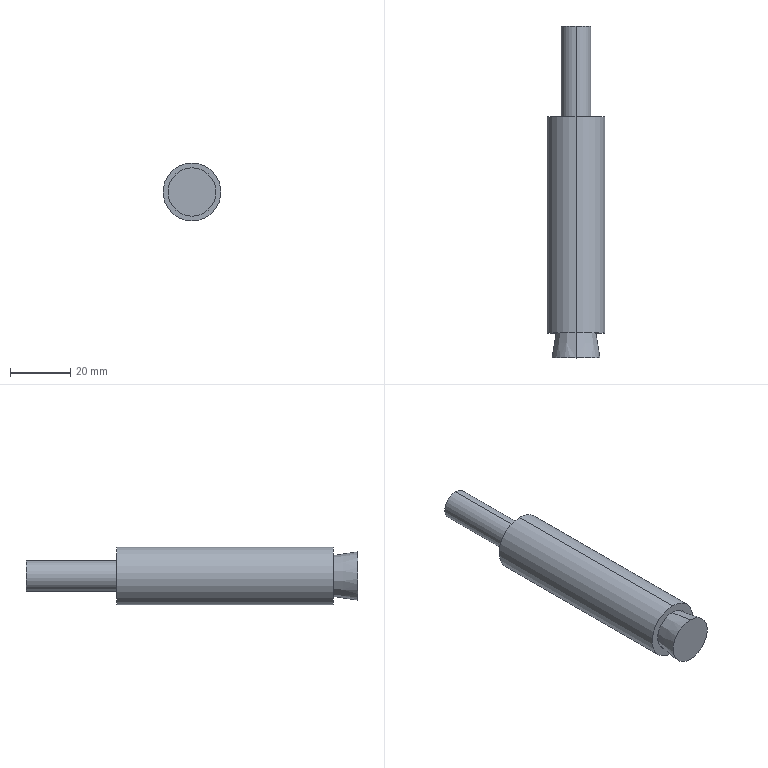Part | STEP file | Expansion Bolt M10X110 | 2 solids | 12 faces | box 19.178 x 110 x 19.178 mm | volume 19450 mm3 | cylinder 6 | plane 4 | cone 2 | commonest cylinder face diameters 10 x2 14 x2 19.178 x2
STEP:
#1=CARTESIAN_POINT('',(0.,0.,0.));
#2=DIRECTION('',(0.,0.,1.));
#3=DIRECTION('',(1.,0.,0.));
#4=AXIS2_PLACEMENT_3D('',#1,#2,#3);
#5=CARTESIAN_POINT('',(0.,110.,-5.));
#6=VERTEX_POINT('',#5);
#7=CARTESIAN_POINT('',(0.,110.,5.));
#8=VERTEX_POINT('',#7);
#9=CARTESIAN_POINT('',(0.,110.,0.));
#10=DIRECTION('',(0.,-1.,0.));
#11=DIRECTION('',(0.,0.,-1.));
#12=AXIS2_PLACEMENT_3D('',#9,#10,#11);
#13=CIRCLE('',#12,5.);
#14=CARTESIAN_POINT('',(0.,0.,0.));
#15=DIRECTION('',(0.,-1.,0.));
#16=DIRECTION('',(0.,0.,-1.));
#17=AXIS2_PLACEMENT_3D('',#14,#15,#16);
#18=CYLINDRICAL_SURFACE('',#17,5.);
#19=CARTESIAN_POINT('',(0.,-110.));
#20=DIRECTION('',(1.,0.));
#21=VECTOR('',#20,1.);
#22=LINE('',#19,#21);
#23=(GEOMETRIC_REPRESENTATION_CONTEXT(2)PARAMETRIC_REPRESENTATION_CONTEXT()REPRESENTATION_CONTEXT('',''));
#24=DEFINITIONAL_REPRESENTATION('',(#22),#23);
#25=PCURVE('',#18,#24);
#26=CARTESIAN_POINT('',(0.,110.,0.));
#27=DIRECTION('',(0.,1.,0.));
#28=DIRECTION('',(0.,0.,1.));
#29=AXIS2_PLACEMENT_3D('',#26,#27,#28);
#30=PLANE('',#29);
#31=CARTESIAN_POINT('',(-5.,0.));
#32=CARTESIAN_POINT('',(-5.,8.66));
#33=CARTESIAN_POINT('',(2.5,4.33));
#34=CARTESIAN_POINT('',(10.,0.));
#35=CARTESIAN_POINT('',(2.5,-4.33));
#36=CARTESIAN_POINT('',(-5.,-8.66));
#37=CARTESIAN_POINT('',(-5.,0.));
#38=(BOUNDED_CURVE()B_SPLINE_CURVE(2,(#31,#32,#33,#34,#35,#36,#37),.UNSPECIFIED.,.T.,.F.)B_SPLINE_CURVE_WITH_KNOTS((1,2,2,2,2,1),(-2.094,0.,2.094,4.189,6.283,8.378),.UNSPECIFIED.)CURVE()GEOMETRIC_REPRESENTATION_ITEM()RATIONAL_B_SPLINE_CURVE((1.,0.5,1.,0.5,1.,0.5,1.))REPRESENTATION_ITEM(''));
#39=(GEOMETRIC_REPRESENTATION_CONTEXT(2)PARAMETRIC_REPRESENTATION_CONTEXT()REPRESENTATION_CONTEXT('',''));
#40=DEFINITIONAL_REPRESENTATION('',(#38),#39);
#41=PCURVE('',#30,#40);
#42=SURFACE_CURVE('',#13,(#25,#41),.PCURVE_S1.);
#43=EDGE_CURVE('',#6,#8,#42,.T.);
#44=ORIENTED_EDGE('',*,*,#43,.T.);
#45=CARTESIAN_POINT('',(0.,20.,5.));
#46=VERTEX_POINT('',#45);
#47=CARTESIAN_POINT('',(0.,0.,5.));
#48=DIRECTION('',(0.,-1.,0.));
#49=VECTOR('',#48,1.);
#50=LINE('',#47,#49);
#51=CARTESIAN_POINT('',(3.142,0.));
#52=DIRECTION('',(0.,1.));
#53=VECTOR('',#52,1.);
#54=LINE('',#51,#53);
#55=(GEOMETRIC_REPRESENTATION_CONTEXT(2)PARAMETRIC_REPRESENTATION_CONTEXT()REPRESENTATION_CONTEXT('',''));
#56=DEFINITIONAL_REPRESENTATION('',(#54),#55);
#57=PCURVE('',#18,#56);
#58=CARTESIAN_POINT('',(0.,0.,0.));
#59=DIRECTION('',(0.,-1.,0.));
#60=DIRECTION('',(0.,0.,-1.));
#61=AXIS2_PLACEMENT_3D('',#58,#59,#60);
#62=CYLINDRICAL_SURFACE('',#61,5.);
#63=CARTESIAN_POINT('',(3.142,0.));
#64=DIRECTION('',(0.,1.));
#65=VECTOR('',#64,1.);
#66=LINE('',#63,#65);
#67=(GEOMETRIC_REPRESENTATION_CONTEXT(2)PARAMETRIC_REPRESENTATION_CONTEXT()REPRESENTATION_CONTEXT('',''));
#68=DEFINITIONAL_REPRESENTATION('',(#66),#67);
#69=PCURVE('',#62,#68);
#70=SURFACE_CURVE('',#50,(#57,#69),.PCURVE_S1.);
#71=EDGE_CURVE('',#8,#46,#70,.T.);
#72=ORIENTED_EDGE('',*,*,#71,.T.);
#73=CARTESIAN_POINT('',(0.,20.,-5.));
#74=VERTEX_POINT('',#73);
#75=CARTESIAN_POINT('',(0.,20.,0.));
#76=DIRECTION('',(0.,-1.,0.));
#77=DIRECTION('',(0.,0.,-1.));
#78=AXIS2_PLACEMENT_3D('',#75,#76,#77);
#79=CIRCLE('',#78,5.);
#80=CARTESIAN_POINT('',(0.,-20.));
#81=DIRECTION('',(1.,0.));
#82=VECTOR('',#81,1.);
#83=LINE('',#80,#82);
#84=(GEOMETRIC_REPRESENTATION_CONTEXT(2)PARAMETRIC_REPRESENTATION_CONTEXT()REPRESENTATION_CONTEXT('',''));
#85=DEFINITIONAL_REPRESENTATION('',(#83),#84);
#86=PCURVE('',#18,#85);
#87=CARTESIAN_POINT('',(0.,0.,0.));
#88=DIRECTION('',(0.,-1.,0.));
#89=DIRECTION('',(0.,0.,-1.));
#90=AXIS2_PLACEMENT_3D('',#87,#88,#89);
#91=CONICAL_SURFACE('',#90,8.,0.1489);
#92=CARTESIAN_POINT('',(0.,-20.));
#93=DIRECTION('',(1.,0.));
#94=VECTOR('',#93,1.);
#95=LINE('',#92,#94);
#96=(GEOMETRIC_REPRESENTATION_CONTEXT(2)PARAMETRIC_REPRESENTATION_CONTEXT()REPRESENTATION_CONTEXT('',''));
#97=DEFINITIONAL_REPRESENTATION('',(#95),#96);
#98=PCURVE('',#91,#97);
#99=SURFACE_CURVE('',#79,(#86,#98),.PCURVE_S1.);
#100=EDGE_CURVE('',#74,#46,#99,.T.);
#101=ORIENTED_EDGE('',*,*,#100,.F.);
#102=CARTESIAN_POINT('',(0.,0.,-5.));
#103=DIRECTION('',(0.,-1.,0.));
#104=VECTOR('',#103,1.);
#105=LINE('',#102,#104);
#106=CARTESIAN_POINT('',(0.,0.));
#107=DIRECTION('',(0.,1.));
#108=VECTOR('',#107,1.);
#109=LINE('',#106,#108);
#110=(GEOMETRIC_REPRESENTATION_CONTEXT(2)PARAMETRIC_REPRESENTATION_CONTEXT()REPRESENTATION_CONTEXT('',''));
#111=DEFINITIONAL_REPRESENTATION('',(#109),#110);
#112=PCURVE('',#18,#111);
#113=CARTESIAN_POINT('',(6.283,0.));
#114=DIRECTION('',(0.,1.));
#115=VECTOR('',#114,1.);
#116=LINE('',#113,#115);
#117=(GEOMETRIC_REPRESENTATION_CONTEXT(2)PARAMETRIC_REPRESENTATION_CONTEXT()REPRESENTATION_CONTEXT('',''));
#118=DEFINITIONAL_REPRESENTATION('',(#116),#117);
#119=PCURVE('',#62,#118);
#120=SURFACE_CURVE('',#105,(#112,#119),.PCURVE_S1.);
#121=EDGE_CURVE('',#6,#74,#120,.T.);
#122=ORIENTED_EDGE('',*,*,#121,.F.);
#123=EDGE_LOOP('',(#44,#72,#101,#122));
#124=FACE_BOUND('',#123,.T.);
#125=ADVANCED_FACE('',(#124),#18,.T.);
#126=ORIENTED_EDGE('',*,*,#100,.T.);
#127=CARTESIAN_POINT('',(0.,0.,8.));
#128=VERTEX_POINT('',#127);
#129=CARTESIAN_POINT('',(0.,0.,8.));
#130=DIRECTION('',(0.,-0.9889,0.1483));
#131=VECTOR('',#130,1.);
#132=LINE('',#129,#131);
#133=CARTESIAN_POINT('',(3.142,0.));
#134=DIRECTION('',(0.,1.));
#135=VECTOR('',#134,1.);
#136=LINE('',#133,#135);
#137=(GEOMETRIC_REPRESENTATION_CONTEXT(2)PARAMETRIC_REPRESENTATION_CONTEXT()REPRESENTATION_CONTEXT('',''));
#138=DEFINITIONAL_REPRESENTATION('',(#136),#137);
#139=PCURVE('',#91,#138);
#140=CARTESIAN_POINT('',(0.,0.,0.));
#141=DIRECTION('',(0.,-1.,0.));
#142=DIRECTION('',(0.,0.,-1.));
#143=AXIS2_PLACEMENT_3D('',#140,#141,#142);
#144=CONICAL_SURFACE('',#143,8.,0.1489);
#145=CARTESIAN_POINT('',(3.142,0.));
#146=DIRECTION('',(0.,1.));
#147=VECTOR('',#146,1.);
#148=LINE('',#145,#147);
#149=(GEOMETRIC_REPRESENTATION_CONTEXT(2)PARAMETRIC_REPRESENTATION_CONTEXT()REPRESENTATION_CONTEXT('',''));
#150=DEFINITIONAL_REPRESENTATION('',(#148),#149);
#151=PCURVE('',#144,#150);
#152=SURFACE_CURVE('',#132,(#139,#151),.PCURVE_S1.);
#153=EDGE_CURVE('',#46,#128,#152,.T.);
#154=ORIENTED_EDGE('',*,*,#153,.T.);
#155=CARTESIAN_POINT('',(0.,0.,-8.));
#156=VERTEX_POINT('',#155);
#157=CARTESIAN_POINT('',(0.,0.,0.));
#158=DIRECTION('',(0.,-1.,0.));
#159=DIRECTION('',(0.,0.,-1.));
#160=AXIS2_PLACEMENT_3D('',#157,#158,#159);
#161=CIRCLE('',#160,8.);
#162=CARTESIAN_POINT('',(0.,0.));
#163=DIRECTION('',(1.,0.));
#164=VECTOR('',#163,1.);
#165=LINE('',#162,#164);
#166=(GEOMETRIC_REPRESENTATION_CONTEXT(2)PARAMETRIC_REPRESENTATION_CONTEXT()REPRESENTATION_CONTEXT('',''));
#167=DEFINITIONAL_REPRESENTATION('',(#165),#166);
#168=PCURVE('',#91,#167);
#169=CARTESIAN_POINT('',(0.,0.,0.));
#170=DIRECTION('',(0.,-1.,0.));
#171=DIRECTION('',(0.,0.,-1.));
#172=AXIS2_PLACEMENT_3D('',#169,#170,#171);
#173=PLANE('',#172);
#174=CARTESIAN_POINT('',(0.,0.));
#175=DIRECTION('',(1.,0.));
#176=AXIS2_PLACEMENT_2D('',#174,#175);
#177=CIRCLE('',#176,8.);
#178=(GEOMETRIC_REPRESENTATION_CONTEXT(2)PARAMETRIC_REPRESENTATION_CONTEXT()REPRESENTATION_CONTEXT('',''));
#179=DEFINITIONAL_REPRESENTATION('',(#177),#178);
#180=PCURVE('',#173,#179);
#181=SURFACE_CURVE('',#161,(#168,#180),.PCURVE_S1.);
#182=EDGE_CURVE('',#156,#128,#181,.T.);
#183=ORIENTED_EDGE('',*,*,#182,.F.);
#184=CARTESIAN_POINT('',(0.,0.,-8.));
#185=DIRECTION('',(0.,-0.9889,-0.1483));
#186=VECTOR('',#185,1.);
#187=LINE('',#184,#186);
#188=CARTESIAN_POINT('',(0.,0.));
#189=DIRECTION('',(0.,1.));
#190=VECTOR('',#189,1.);
#191=LINE('',#188,#190);
#192=(GEOMETRIC_REPRESENTATION_CONTEXT(2)PARAMETRIC_REPRESENTATION_CONTEXT()REPRESENTATION_CONTEXT('',''));
#193=DEFINITIONAL_REPRESENTATION('',(#191),#192);
#194=PCURVE('',#91,#193);
#195=CARTESIAN_POINT('',(6.283,0.));
#196=DIRECTION('',(0.,1.));
#197=VECTOR('',#196,1.);
#198=LINE('',#195,#197);
#199=(GEOMETRIC_REPRESENTATION_CONTEXT(2)PARAMETRIC_REPRESENTATION_CONTEXT()REPRESENTATION_CONTEXT('',''));
#200=DEFINITIONAL_REPRESENTATION('',(#198),#199);
#201=PCURVE('',#144,#200);
#202=SURFACE_CURVE('',#187,(#194,#201),.PCURVE_S1.);
#203=EDGE_CURVE('',#74,#156,#202,.T.);
#204=ORIENTED_EDGE('',*,*,#203,.F.);
#205=EDGE_LOOP('',(#126,#154,#183,#204));
#206=FACE_BOUND('',#205,.T.);
#207=ADVANCED_FACE('',(#206),#91,.T.);
#208=ORIENTED_EDGE('',*,*,#182,.T.);
#209=CARTESIAN_POINT('',(0.,0.,0.));
#210=DIRECTION('',(0.,-1.,0.));
#211=DIRECTION('',(0.,0.,-1.));
#212=AXIS2_PLACEMENT_3D('',#209,#210,#211);
#213=CIRCLE('',#212,8.);
#214=CARTESIAN_POINT('',(0.,0.));
#215=DIRECTION('',(1.,0.));
#216=AXIS2_PLACEMENT_2D('',#214,#215);
#217=CIRCLE('',#216,8.);
#218=(GEOMETRIC_REPRESENTATION_CONTEXT(2)PARAMETRIC_REPRESENTATION_CONTEXT()REPRESENTATION_CONTEXT('',''));
#219=DEFINITIONAL_REPRESENTATION('',(#217),#218);
#220=PCURVE('',#173,#219);
#221=CARTESIAN_POINT('',(0.,0.));
#222=DIRECTION('',(1.,0.));
#223=VECTOR('',#222,1.);
#224=LINE('',#221,#223);
#225=(GEOMETRIC_REPRESENTATION_CONTEXT(2)PARAMETRIC_REPRESENTATION_CONTEXT()REPRESENTATION_CONTEXT('',''));
#226=DEFINITIONAL_REPRESENTATION('',(#224),#225);
#227=PCURVE('',#144,#226);
#228=SURFACE_CURVE('',#213,(#220,#227),.PCURVE_S1.);
#229=EDGE_CURVE('',#128,#156,#228,.T.);
#230=ORIENTED_EDGE('',*,*,#229,.T.);
#231=EDGE_LOOP('',(#208,#230));
#232=FACE_BOUND('',#231,.T.);
#233=ADVANCED_FACE('',(#232),#173,.T.);
#234=ORIENTED_EDGE('',*,*,#153,.F.);
#235=CARTESIAN_POINT('',(0.,20.,0.));
#236=DIRECTION('',(0.,-1.,0.));
#237=DIRECTION('',(0.,0.,-1.));
#238=AXIS2_PLACEMENT_3D('',#235,#236,#237);
#239=CIRCLE('',#238,5.);
#240=CARTESIAN_POINT('',(0.,-20.));
#241=DIRECTION('',(1.,0.));
#242=VECTOR('',#241,1.);
#243=LINE('',#240,#242);
#244=(GEOMETRIC_REPRESENTATION_CONTEXT(2)PARAMETRIC_REPRESENTATION_CONTEXT()REPRESENTATION_CONTEXT('',''));
#245=DEFINITIONAL_REPRESENTATION('',(#243),#244);
#246=PCURVE('',#144,#245);
#247=CARTESIAN_POINT('',(0.,-20.));
#248=DIRECTION('',(1.,0.));
#249=VECTOR('',#248,1.);
#250=LINE('',#247,#249);
#251=(GEOMETRIC_REPRESENTATION_CONTEXT(2)PARAMETRIC_REPRESENTATION_CONTEXT()REPRESENTATION_CONTEXT('',''));
#252=DEFINITIONAL_REPRESENTATION('',(#250),#251);
#253=PCURVE('',#62,#252);
#254=SURFACE_CURVE('',#239,(#246,#253),.PCURVE_S1.);
#255=EDGE_CURVE('',#46,#74,#254,.T.);
#256=ORIENTED_EDGE('',*,*,#255,.T.);
#257=ORIENTED_EDGE('',*,*,#203,.T.);
#258=ORIENTED_EDGE('',*,*,#229,.F.);
#259=EDGE_LOOP('',(#234,#256,#257,#258));
#260=FACE_BOUND('',#259,.T.);
#261=ADVANCED_FACE('',(#260),#144,.T.);
#262=ORIENTED_EDGE('',*,*,#71,.F.);
#263=CARTESIAN_POINT('',(0.,110.,0.));
#264=DIRECTION('',(0.,-1.,0.));
#265=DIRECTION('',(0.,0.,-1.));
#266=AXIS2_PLACEMENT_3D('',#263,#264,#265);
#267=CIRCLE('',#266,5.);
#268=CARTESIAN_POINT('',(0.,-110.));
#269=DIRECTION('',(1.,0.));
#270=VECTOR('',#269,1.);
#271=LINE('',#268,#270);
#272=(GEOMETRIC_REPRESENTATION_CONTEXT(2)PARAMETRIC_REPRESENTATION_CONTEXT()REPRESENTATION_CONTEXT('',''));
#273=DEFINITIONAL_REPRESENTATION('',(#271),#272);
#274=PCURVE('',#62,#273);
#275=CARTESIAN_POINT('',(-5.,0.));
#276=CARTESIAN_POINT('',(-5.,8.66));
#277=CARTESIAN_POINT('',(2.5,4.33));
#278=CARTESIAN_POINT('',(10.,0.));
#279=CARTESIAN_POINT('',(2.5,-4.33));
#280=CARTESIAN_POINT('',(-5.,-8.66));
#281=CARTESIAN_POINT('',(-5.,0.));
#282=(BOUNDED_CURVE()B_SPLINE_CURVE(2,(#275,#276,#277,#278,#279,#280,#281),.UNSPECIFIED.,.T.,.F.)B_SPLINE_CURVE_WITH_KNOTS((1,2,2,2,2,1),(-2.094,0.,2.094,4.189,6.283,8.378),.UNSPECIFIED.)CURVE()GEOMETRIC_REPRESENTATION_ITEM()RATIONAL_B_SPLINE_CURVE((1.,0.5,1.,0.5,1.,0.5,1.))REPRESENTATION_ITEM(''));
#283=(GEOMETRIC_REPRESENTATION_CONTEXT(2)PARAMETRIC_REPRESENTATION_CONTEXT()REPRESENTATION_CONTEXT('',''));
#284=DEFINITIONAL_REPRESENTATION('',(#282),#283);
#285=PCURVE('',#30,#284);
#286=SURFACE_CURVE('',#267,(#274,#285),.PCURVE_S1.);
#287=EDGE_CURVE('',#8,#6,#286,.T.);
#288=ORIENTED_EDGE('',*,*,#287,.T.);
#289=ORIENTED_EDGE('',*,*,#121,.T.);
#290=ORIENTED_EDGE('',*,*,#255,.F.);
#291=EDGE_LOOP('',(#262,#288,#289,#290));
#292=FACE_BOUND('',#291,.T.);
#293=ADVANCED_FACE('',(#292),#62,.T.);
#294=ORIENTED_EDGE('',*,*,#43,.F.);
#295=ORIENTED_EDGE('',*,*,#287,.F.);
#296=EDGE_LOOP('',(#294,#295));
#297=FACE_BOUND('',#296,.T.);
#298=ADVANCED_FACE('',(#297),#30,.T.);
#299=CLOSED_SHELL('',(#125,#207,#233,#261,#293,#298));
#300=MANIFOLD_SOLID_BREP('',#299);
#301=CARTESIAN_POINT('',(0.,80.,-7.));
#302=VERTEX_POINT('',#301);
#303=CARTESIAN_POINT('',(0.,8.265,-7.));
#304=VERTEX_POINT('',#303);
#305=CARTESIAN_POINT('',(0.,0.,-7.));
#306=DIRECTION('',(0.,-1.,0.));
#307=VECTOR('',#306,1.);
#308=LINE('',#305,#307);
#309=CARTESIAN_POINT('',(0.,0.,0.));
#310=DIRECTION('',(0.,-1.,0.));
#311=DIRECTION('',(0.,0.,-1.));
#312=AXIS2_PLACEMENT_3D('',#309,#310,#311);
#313=CYLINDRICAL_SURFACE('',#312,7.);
#314=CARTESIAN_POINT('',(6.283,0.));
#315=DIRECTION('',(0.,1.));
#316=VECTOR('',#315,1.);
#317=LINE('',#314,#316);
#318=(GEOMETRIC_REPRESENTATION_CONTEXT(2)PARAMETRIC_REPRESENTATION_CONTEXT()REPRESENTATION_CONTEXT('',''));
#319=DEFINITIONAL_REPRESENTATION('',(#317),#318);
#320=PCURVE('',#313,#319);
#321=CARTESIAN_POINT('',(0.,0.,0.));
#322=DIRECTION('',(0.,-1.,0.));
#323=DIRECTION('',(0.,0.,-1.));
#324=AXIS2_PLACEMENT_3D('',#321,#322,#323);
#325=CYLINDRICAL_SURFACE('',#324,7.);
#326=CARTESIAN_POINT('',(0.,0.));
#327=DIRECTION('',(0.,1.));
#328=VECTOR('',#327,1.);
#329=LINE('',#326,#328);
#330=(GEOMETRIC_REPRESENTATION_CONTEXT(2)PARAMETRIC_REPRESENTATION_CONTEXT()REPRESENTATION_CONTEXT('',''));
#331=DEFINITIONAL_REPRESENTATION('',(#329),#330);
#332=PCURVE('',#325,#331);
#333=SURFACE_CURVE('',#308,(#320,#332),.PCURVE_S1.);
#334=EDGE_CURVE('',#302,#304,#333,.T.);
#335=ORIENTED_EDGE('',*,*,#334,.T.);
#336=CARTESIAN_POINT('',(0.,8.265,7.));
#337=VERTEX_POINT('',#336);
#338=CARTESIAN_POINT('',(0.,8.265,0.));
#339=DIRECTION('',(0.,-1.,0.));
#340=DIRECTION('',(0.,0.,-1.));
#341=AXIS2_PLACEMENT_3D('',#338,#339,#340);
#342=CIRCLE('',#341,7.);
#343=CARTESIAN_POINT('',(0.,-8.265));
#344=DIRECTION('',(1.,0.));
#345=VECTOR('',#344,1.);
#346=LINE('',#343,#345);
#347=(GEOMETRIC_REPRESENTATION_CONTEXT(2)PARAMETRIC_REPRESENTATION_CONTEXT()REPRESENTATION_CONTEXT('',''));
#348=DEFINITIONAL_REPRESENTATION('',(#346),#347);
#349=PCURVE('',#313,#348);
#350=CARTESIAN_POINT('',(7.,8.265,0.));
#351=DIRECTION('',(0.,-1.,0.));
#352=DIRECTION('',(0.,0.,-1.));
#353=AXIS2_PLACEMENT_3D('',#350,#351,#352);
#354=PLANE('',#353);
#355=CARTESIAN_POINT('',(0.,-7.));
#356=DIRECTION('',(1.,0.));
#357=AXIS2_PLACEMENT_2D('',#355,#356);
#358=CIRCLE('',#357,7.);
#359=(GEOMETRIC_REPRESENTATION_CONTEXT(2)PARAMETRIC_REPRESENTATION_CONTEXT()REPRESENTATION_CONTEXT('',''));
#360=DEFINITIONAL_REPRESENTATION('',(#358),#359);
#361=PCURVE('',#354,#360);
#362=SURFACE_CURVE('',#342,(#349,#361),.PCURVE_S1.);
#363=EDGE_CURVE('',#337,#304,#362,.T.);
#364=ORIENTED_EDGE('',*,*,#363,.F.);
#365=CARTESIAN_POINT('',(0.,80.,7.));
#366=VERTEX_POINT('',#365);
#367=CARTESIAN_POINT('',(0.,0.,7.));
#368=DIRECTION('',(0.,-1.,0.));
#369=VECTOR('',#368,1.);
#370=LINE('',#367,#369);
#371=CARTESIAN_POINT('',(3.142,0.));
#372=DIRECTION('',(0.,1.));
#373=VECTOR('',#372,1.);
#374=LINE('',#371,#373);
#375=(GEOMETRIC_REPRESENTATION_CONTEXT(2)PARAMETRIC_REPRESENTATION_CONTEXT()REPRESENTATION_CONTEXT('',''));
#376=DEFINITIONAL_REPRESENTATION('',(#374),#375);
#377=PCURVE('',#313,#376);
#378=CARTESIAN_POINT('',(3.142,0.));
#379=DIRECTION('',(0.,1.));
#380=VECTOR('',#379,1.);
#381=LINE('',#378,#380);
#382=(GEOMETRIC_REPRESENTATION_CONTEXT(2)PARAMETRIC_REPRESENTATION_CONTEXT()REPRESENTATION_CONTEXT('',''));
#383=DEFINITIONAL_REPRESENTATION('',(#381),#382);
#384=PCURVE('',#325,#383);
#385=SURFACE_CURVE('',#370,(#377,#384),.PCURVE_S1.);
#386=EDGE_CURVE('',#366,#337,#385,.T.);
#387=ORIENTED_EDGE('',*,*,#386,.F.);
#388=CARTESIAN_POINT('',(0.,80.,0.));
#389=DIRECTION('',(0.,-1.,0.));
#390=DIRECTION('',(0.,0.,-1.));
#391=AXIS2_PLACEMENT_3D('',#388,#389,#390);
#392=CIRCLE('',#391,7.);
#393=CARTESIAN_POINT('',(0.,-80.));
#394=DIRECTION('',(1.,0.));
#395=VECTOR('',#394,1.);
#396=LINE('',#393,#395);
#397=(GEOMETRIC_REPRESENTATION_CONTEXT(2)PARAMETRIC_REPRESENTATION_CONTEXT()REPRESENTATION_CONTEXT('',''));
#398=DEFINITIONAL_REPRESENTATION('',(#396),#397);
#399=PCURVE('',#313,#398);
#400=CARTESIAN_POINT('',(9.589,80.,0.));
#401=DIRECTION('',(0.,1.,0.));
#402=DIRECTION('',(0.,0.,1.));
#403=AXIS2_PLACEMENT_3D('',#400,#401,#402);
#404=PLANE('',#403);
#405=CARTESIAN_POINT('',(-7.,-9.589));
#406=CARTESIAN_POINT('',(-7.,2.535));
#407=CARTESIAN_POINT('',(3.5,-3.527));
#408=CARTESIAN_POINT('',(14.,-9.589));
#409=CARTESIAN_POINT('',(3.5,-15.651));
#410=CARTESIAN_POINT('',(-7.,-21.714));
#411=CARTESIAN_POINT('',(-7.,-9.589));
#412=(BOUNDED_CURVE()B_SPLINE_CURVE(2,(#405,#406,#407,#408,#409,#410,#411),.UNSPECIFIED.,.T.,.F.)B_SPLINE_CURVE_WITH_KNOTS((1,2,2,2,2,1),(-2.094,0.,2.094,4.189,6.283,8.378),.UNSPECIFIED.)CURVE()GEOMETRIC_REPRESENTATION_ITEM()RATIONAL_B_SPLINE_CURVE((1.,0.5,1.,0.5,1.,0.5,1.))REPRESENTATION_ITEM(''));
#413=(GEOMETRIC_REPRESENTATION_CONTEXT(2)PARAMETRIC_REPRESENTATION_CONTEXT()REPRESENTATION_CONTEXT('',''));
#414=DEFINITIONAL_REPRESENTATION('',(#412),#413);
#415=PCURVE('',#404,#414);
#416=SURFACE_CURVE('',#392,(#399,#415),.PCURVE_S1.);
#417=EDGE_CURVE('',#366,#302,#416,.T.);
#418=ORIENTED_EDGE('',*,*,#417,.T.);
#419=EDGE_LOOP('',(#335,#364,#387,#418));
#420=FACE_BOUND('',#419,.F.);
#421=ADVANCED_FACE('',(#420),#313,.F.);
#422=CARTESIAN_POINT('',(0.,80.,-9.589));
#423=VERTEX_POINT('',#422);
#424=CARTESIAN_POINT('',(0.,80.,9.589));
#425=VERTEX_POINT('',#424);
#426=CARTESIAN_POINT('',(0.,80.,0.));
#427=DIRECTION('',(0.,-1.,0.));
#428=DIRECTION('',(0.,0.,-1.));
#429=AXIS2_PLACEMENT_3D('',#426,#427,#428);
#430=CIRCLE('',#429,9.589);
#431=CARTESIAN_POINT('',(0.,0.,0.));
#432=DIRECTION('',(0.,-1.,0.));
#433=DIRECTION('',(0.,0.,-1.));
#434=AXIS2_PLACEMENT_3D('',#431,#432,#433);
#435=CYLINDRICAL_SURFACE('',#434,9.589);
#436=CARTESIAN_POINT('',(0.,-80.));
#437=DIRECTION('',(1.,0.));
#438=VECTOR('',#437,1.);
#439=LINE('',#436,#438);
#440=(GEOMETRIC_REPRESENTATION_CONTEXT(2)PARAMETRIC_REPRESENTATION_CONTEXT()REPRESENTATION_CONTEXT('',''));
#441=DEFINITIONAL_REPRESENTATION('',(#439),#440);
#442=PCURVE('',#435,#441);
#443=CARTESIAN_POINT('',(-9.589,-9.589));
#444=CARTESIAN_POINT('',(-9.589,7.02));
#445=CARTESIAN_POINT('',(4.795,-1.285));
#446=CARTESIAN_POINT('',(19.178,-9.589));
#447=CARTESIAN_POINT('',(4.795,-17.894));
#448=CARTESIAN_POINT('',(-9.589,-26.198));
#449=CARTESIAN_POINT('',(-9.589,-9.589));
#450=(BOUNDED_CURVE()B_SPLINE_CURVE(2,(#443,#444,#445,#446,#447,#448,#449),.UNSPECIFIED.,.T.,.F.)B_SPLINE_CURVE_WITH_KNOTS((1,2,2,2,2,1),(-2.094,0.,2.094,4.189,6.283,8.378),.UNSPECIFIED.)CURVE()GEOMETRIC_REPRESENTATION_ITEM()RATIONAL_B_SPLINE_CURVE((1.,0.5,1.,0.5,1.,0.5,1.))REPRESENTATION_ITEM(''));
#451=(GEOMETRIC_REPRESENTATION_CONTEXT(2)PARAMETRIC_REPRESENTATION_CONTEXT()REPRESENTATION_CONTEXT('',''));
#452=DEFINITIONAL_REPRESENTATION('',(#450),#451);
#453=PCURVE('',#404,#452);
#454=SURFACE_CURVE('',#430,(#442,#453),.PCURVE_S1.);
#455=EDGE_CURVE('',#423,#425,#454,.T.);
#456=ORIENTED_EDGE('',*,*,#455,.T.);
#457=CARTESIAN_POINT('',(0.,8.265,9.589));
#458=VERTEX_POINT('',#457);
#459=CARTESIAN_POINT('',(0.,0.,9.589));
#460=DIRECTION('',(0.,-1.,0.));
#461=VECTOR('',#460,1.);
#462=LINE('',#459,#461);
#463=CARTESIAN_POINT('',(3.142,0.));
#464=DIRECTION('',(0.,1.));
#465=VECTOR('',#464,1.);
#466=LINE('',#463,#465);
#467=(GEOMETRIC_REPRESENTATION_CONTEXT(2)PARAMETRIC_REPRESENTATION_CONTEXT()REPRESENTATION_CONTEXT('',''));
#468=DEFINITIONAL_REPRESENTATION('',(#466),#467);
#469=PCURVE('',#435,#468);
#470=CARTESIAN_POINT('',(0.,0.,0.));
#471=DIRECTION('',(0.,-1.,0.));
#472=DIRECTION('',(0.,0.,-1.));
#473=AXIS2_PLACEMENT_3D('',#470,#471,#472);
#474=CYLINDRICAL_SURFACE('',#473,9.589);
#475=CARTESIAN_POINT('',(3.142,0.));
#476=DIRECTION('',(0.,1.));
#477=VECTOR('',#476,1.);
#478=LINE('',#475,#477);
#479=(GEOMETRIC_REPRESENTATION_CONTEXT(2)PARAMETRIC_REPRESENTATION_CONTEXT()REPRESENTATION_CONTEXT('',''));
#480=DEFINITIONAL_REPRESENTATION('',(#478),#479);
#481=PCURVE('',#474,#480);
#482=SURFACE_CURVE('',#462,(#469,#481),.PCURVE_S1.);
#483=EDGE_CURVE('',#425,#458,#482,.T.);
#484=ORIENTED_EDGE('',*,*,#483,.T.);
#485=CARTESIAN_POINT('',(0.,8.265,-9.589));
#486=VERTEX_POINT('',#485);
#487=CARTESIAN_POINT('',(0.,8.265,0.));
#488=DIRECTION('',(0.,-1.,0.));
#489=DIRECTION('',(0.,0.,-1.));
#490=AXIS2_PLACEMENT_3D('',#487,#488,#489);
#491=CIRCLE('',#490,9.589);
#492=CARTESIAN_POINT('',(0.,-8.265));
#493=DIRECTION('',(1.,0.));
#494=VECTOR('',#493,1.);
#495=LINE('',#492,#494);
#496=(GEOMETRIC_REPRESENTATION_CONTEXT(2)PARAMETRIC_REPRESENTATION_CONTEXT()REPRESENTATION_CONTEXT('',''));
#497=DEFINITIONAL_REPRESENTATION('',(#495),#496);
#498=PCURVE('',#435,#497);
#499=CARTESIAN_POINT('',(0.,-7.));
#500=DIRECTION('',(1.,0.));
#501=AXIS2_PLACEMENT_2D('',#499,#500);
#502=CIRCLE('',#501,9.589);
#503=(GEOMETRIC_REPRESENTATION_CONTEXT(2)PARAMETRIC_REPRESENTATION_CONTEXT()REPRESENTATION_CONTEXT('',''));
#504=DEFINITIONAL_REPRESENTATION('',(#502),#503);
#505=PCURVE('',#354,#504);
#506=SURFACE_CURVE('',#491,(#498,#505),.PCURVE_S1.);
#507=EDGE_CURVE('',#486,#458,#506,.T.);
#508=ORIENTED_EDGE('',*,*,#507,.F.);
#509=CARTESIAN_POINT('',(0.,0.,-9.589));
#510=DIRECTION('',(0.,-1.,0.));
#511=VECTOR('',#510,1.);
#512=LINE('',#509,#511);
#513=CARTESIAN_POINT('',(0.,0.));
#514=DIRECTION('',(0.,1.));
#515=VECTOR('',#514,1.);
#516=LINE('',#513,#515);
#517=(GEOMETRIC_REPRESENTATION_CONTEXT(2)PARAMETRIC_REPRESENTATION_CONTEXT()REPRESENTATION_CONTEXT('',''));
#518=DEFINITIONAL_REPRESENTATION('',(#516),#517);
#519=PCURVE('',#435,#518);
#520=CARTESIAN_POINT('',(6.283,0.));
#521=DIRECTION('',(0.,1.));
#522=VECTOR('',#521,1.);
#523=LINE('',#520,#522);
#524=(GEOMETRIC_REPRESENTATION_CONTEXT(2)PARAMETRIC_REPRESENTATION_CONTEXT()REPRESENTATION_CONTEXT('',''));
#525=DEFINITIONAL_REPRESENTATION('',(#523),#524);
#526=PCURVE('',#474,#525);
#527=SURFACE_CURVE('',#512,(#519,#526),.PCURVE_S1.);
#528=EDGE_CURVE('',#423,#486,#527,.T.);
#529=ORIENTED_EDGE('',*,*,#528,.F.);
#530=EDGE_LOOP('',(#456,#484,#508,#529));
#531=FACE_BOUND('',#530,.T.);
#532=ADVANCED_FACE('',(#531),#435,.T.);
#533=ORIENTED_EDGE('',*,*,#507,.T.);
#534=CARTESIAN_POINT('',(0.,8.265,0.));
#535=DIRECTION('',(0.,-1.,0.));
#536=DIRECTION('',(0.,0.,-1.));
#537=AXIS2_PLACEMENT_3D('',#534,#535,#536);
#538=CIRCLE('',#537,9.589);
#539=CARTESIAN_POINT('',(0.,-7.));
#540=DIRECTION('',(1.,0.));
#541=AXIS2_PLACEMENT_2D('',#539,#540);
#542=CIRCLE('',#541,9.589);
#543=(GEOMETRIC_REPRESENTATION_CONTEXT(2)PARAMETRIC_REPRESENTATION_CONTEXT()REPRESENTATION_CONTEXT('',''));
#544=DEFINITIONAL_REPRESENTATION('',(#542),#543);
#545=PCURVE('',#354,#544);
#546=CARTESIAN_POINT('',(0.,-8.265));
#547=DIRECTION('',(1.,0.));
#548=VECTOR('',#547,1.);
#549=LINE('',#546,#548);
#550=(GEOMETRIC_REPRESENTATION_CONTEXT(2)PARAMETRIC_REPRESENTATION_CONTEXT()REPRESENTATION_CONTEXT('',''));
#551=DEFINITIONAL_REPRESENTATION('',(#549),#550);
#552=PCURVE('',#474,#551);
#553=SURFACE_CURVE('',#538,(#545,#552),.PCURVE_S1.);
#554=EDGE_CURVE('',#458,#486,#553,.T.);
#555=ORIENTED_EDGE('',*,*,#554,.T.);
#556=EDGE_LOOP('',(#533,#555));
#557=FACE_BOUND('',#556,.T.);
#558=CARTESIAN_POINT('',(0.,8.265,0.));
#559=DIRECTION('',(0.,-1.,0.));
#560=DIRECTION('',(0.,0.,-1.));
#561=AXIS2_PLACEMENT_3D('',#558,#559,#560);
#562=CIRCLE('',#561,7.);
#563=CARTESIAN_POINT('',(0.,-7.));
#564=DIRECTION('',(1.,0.));
#565=AXIS2_PLACEMENT_2D('',#563,#564);
#566=CIRCLE('',#565,7.);
#567=(GEOMETRIC_REPRESENTATION_CONTEXT(2)PARAMETRIC_REPRESENTATION_CONTEXT()REPRESENTATION_CONTEXT('',''));
#568=DEFINITIONAL_REPRESENTATION('',(#566),#567);
#569=PCURVE('',#354,#568);
#570=CARTESIAN_POINT('',(0.,-8.265));
#571=DIRECTION('',(1.,0.));
#572=VECTOR('',#571,1.);
#573=LINE('',#570,#572);
#574=(GEOMETRIC_REPRESENTATION_CONTEXT(2)PARAMETRIC_REPRESENTATION_CONTEXT()REPRESENTATION_CONTEXT('',''));
#575=DEFINITIONAL_REPRESENTATION('',(#573),#574);
#576=PCURVE('',#325,#575);
#577=SURFACE_CURVE('',#562,(#569,#576),.PCURVE_S1.);
#578=EDGE_CURVE('',#304,#337,#577,.T.);
#579=ORIENTED_EDGE('',*,*,#578,.F.);
#580=ORIENTED_EDGE('',*,*,#363,.F.);
#581=EDGE_LOOP('',(#579,#580));
#582=FACE_BOUND('',#581,.T.);
#583=ADVANCED_FACE('',(#557,#582),#354,.T.);
#584=ORIENTED_EDGE('',*,*,#483,.F.);
#585=CARTESIAN_POINT('',(0.,80.,0.));
#586=DIRECTION('',(0.,-1.,0.));
#587=DIRECTION('',(0.,0.,-1.));
#588=AXIS2_PLACEMENT_3D('',#585,#586,#587);
#589=CIRCLE('',#588,9.589);
#590=CARTESIAN_POINT('',(0.,-80.));
#591=DIRECTION('',(1.,0.));
#592=VECTOR('',#591,1.);
#593=LINE('',#590,#592);
#594=(GEOMETRIC_REPRESENTATION_CONTEXT(2)PARAMETRIC_REPRESENTATION_CONTEXT()REPRESENTATION_CONTEXT('',''));
#595=DEFINITIONAL_REPRESENTATION('',(#593),#594);
#596=PCURVE('',#474,#595);
#597=CARTESIAN_POINT('',(-9.589,-9.589));
#598=CARTESIAN_POINT('',(-9.589,7.02));
#599=CARTESIAN_POINT('',(4.795,-1.285));
#600=CARTESIAN_POINT('',(19.178,-9.589));
#601=CARTESIAN_POINT('',(4.795,-17.894));
#602=CARTESIAN_POINT('',(-9.589,-26.198));
#603=CARTESIAN_POINT('',(-9.589,-9.589));
#604=(BOUNDED_CURVE()B_SPLINE_CURVE(2,(#597,#598,#599,#600,#601,#602,#603),.UNSPECIFIED.,.T.,.F.)B_SPLINE_CURVE_WITH_KNOTS((1,2,2,2,2,1),(-2.094,0.,2.094,4.189,6.283,8.378),.UNSPECIFIED.)CURVE()GEOMETRIC_REPRESENTATION_ITEM()RATIONAL_B_SPLINE_CURVE((1.,0.5,1.,0.5,1.,0.5,1.))REPRESENTATION_ITEM(''));
#605=(GEOMETRIC_REPRESENTATION_CONTEXT(2)PARAMETRIC_REPRESENTATION_CONTEXT()REPRESENTATION_CONTEXT('',''));
#606=DEFINITIONAL_REPRESENTATION('',(#604),#605);
#607=PCURVE('',#404,#606);
#608=SURFACE_CURVE('',#589,(#596,#607),.PCURVE_S1.);
#609=EDGE_CURVE('',#425,#423,#608,.T.);
#610=ORIENTED_EDGE('',*,*,#609,.T.);
#611=ORIENTED_EDGE('',*,*,#528,.T.);
#612=ORIENTED_EDGE('',*,*,#554,.F.);
#613=EDGE_LOOP('',(#584,#610,#611,#612));
#614=FACE_BOUND('',#613,.T.);
#615=ADVANCED_FACE('',(#614),#474,.T.);
#616=CARTESIAN_POINT('',(0.,80.,0.));
#617=DIRECTION('',(0.,-1.,0.));
#618=DIRECTION('',(0.,0.,-1.));
#619=AXIS2_PLACEMENT_3D('',#616,#617,#618);
#620=CIRCLE('',#619,7.);
#621=CARTESIAN_POINT('',(-7.,-9.589));
#622=CARTESIAN_POINT('',(-7.,2.535));
#623=CARTESIAN_POINT('',(3.5,-3.527));
#624=CARTESIAN_POINT('',(14.,-9.589));
#625=CARTESIAN_POINT('',(3.5,-15.651));
#626=CARTESIAN_POINT('',(-7.,-21.714));
#627=CARTESIAN_POINT('',(-7.,-9.589));
#628=(BOUNDED_CURVE()B_SPLINE_CURVE(2,(#621,#622,#623,#624,#625,#626,#627),.UNSPECIFIED.,.T.,.F.)B_SPLINE_CURVE_WITH_KNOTS((1,2,2,2,2,1),(-2.094,0.,2.094,4.189,6.283,8.378),.UNSPECIFIED.)CURVE()GEOMETRIC_REPRESENTATION_ITEM()RATIONAL_B_SPLINE_CURVE((1.,0.5,1.,0.5,1.,0.5,1.))REPRESENTATION_ITEM(''));
#629=(GEOMETRIC_REPRESENTATION_CONTEXT(2)PARAMETRIC_REPRESENTATION_CONTEXT()REPRESENTATION_CONTEXT('',''));
#630=DEFINITIONAL_REPRESENTATION('',(#628),#629);
#631=PCURVE('',#404,#630);
#632=CARTESIAN_POINT('',(0.,-80.));
#633=DIRECTION('',(1.,0.));
#634=VECTOR('',#633,1.);
#635=LINE('',#632,#634);
#636=(GEOMETRIC_REPRESENTATION_CONTEXT(2)PARAMETRIC_REPRESENTATION_CONTEXT()REPRESENTATION_CONTEXT('',''));
#637=DEFINITIONAL_REPRESENTATION('',(#635),#636);
#638=PCURVE('',#325,#637);
#639=SURFACE_CURVE('',#620,(#631,#638),.PCURVE_S1.);
#640=EDGE_CURVE('',#302,#366,#639,.T.);
#641=ORIENTED_EDGE('',*,*,#640,.T.);
#642=ORIENTED_EDGE('',*,*,#417,.T.);
#643=EDGE_LOOP('',(#641,#642));
#644=FACE_BOUND('',#643,.T.);
#645=ORIENTED_EDGE('',*,*,#455,.F.);
#646=ORIENTED_EDGE('',*,*,#609,.F.);
#647=EDGE_LOOP('',(#645,#646));
#648=FACE_BOUND('',#647,.T.);
#649=ADVANCED_FACE('',(#644,#648),#404,.T.);
#650=ORIENTED_EDGE('',*,*,#578,.F.);
#651=ORIENTED_EDGE('',*,*,#334,.F.);
#652=ORIENTED_EDGE('',*,*,#640,.T.);
#653=ORIENTED_EDGE('',*,*,#386,.T.);
#654=EDGE_LOOP('',(#650,#651,#652,#653));
#655=FACE_BOUND('',#654,.F.);
#656=ADVANCED_FACE('',(#655),#325,.F.);
#657=CLOSED_SHELL('',(#421,#532,#583,#615,#649,#656));
#658=MANIFOLD_SOLID_BREP('',#657);
#659=(LENGTH_UNIT()NAMED_UNIT(*)SI_UNIT(.MILLI.,.METRE.));
#660=UNCERTAINTY_MEASURE_WITH_UNIT(LENGTH_MEASURE(0.0000001),#659,'','');
#661=(NAMED_UNIT(*)PLANE_ANGLE_UNIT()SI_UNIT($,.RADIAN.));
#662=(NAMED_UNIT(*)SI_UNIT($,.STERADIAN.)SOLID_ANGLE_UNIT());
#663=(GEOMETRIC_REPRESENTATION_CONTEXT(3)GLOBAL_UNCERTAINTY_ASSIGNED_CONTEXT((#660))GLOBAL_UNIT_ASSIGNED_CONTEXT((#659,#661,#662))REPRESENTATION_CONTEXT('',''));
#664=SHAPE_REPRESENTATION('',(#4,#300,#658),#663);